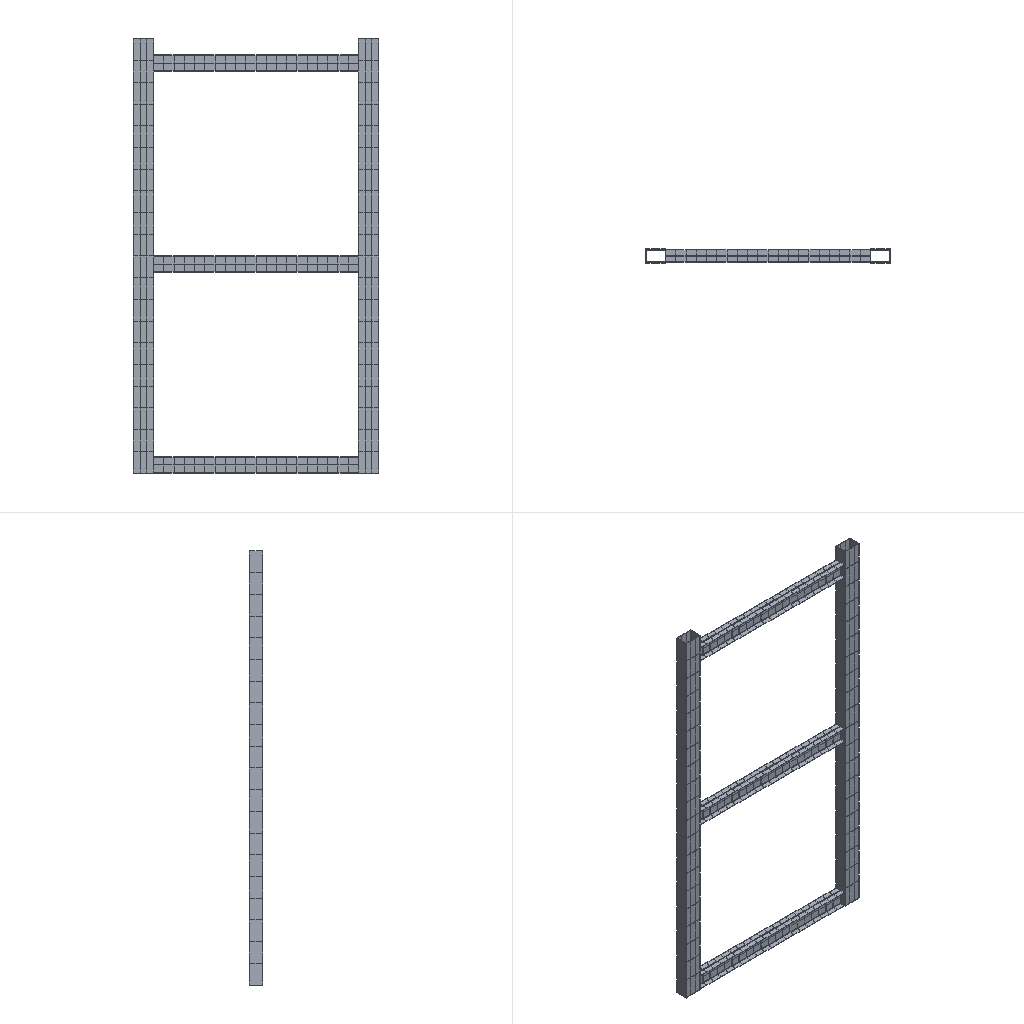Simulation study | abaqus
Set-up summary:
category,name,step,type,value,unit,region
solver,abaqus,,Abaqus/CAE 2024
units,mm-N-s-tonne (MPa),,inferred,E=206000 density=7.85e-09
analysis,Step-1,,static,nlgeom=True; time_period=20
mesh,nodes,,,1807
mesh,elements,,,800
element_type,C3D8R,,,800
material,q335b,,E,206000
material,q335b,,nu,0.3
material,q335b,,density,7.85e-09
material,q335b,,yield,335
material,q335b,,behaviors,plastic
section,q335b,,solid section,,,Set-1
section,q335b,,solid section,,,Set-1
bc,BC-1,initial,encastre,[dofs=ENCASTRE],,_PickedSet31
bc,BC-2,Step-1,displacement,1 [dofs=x],,_PickedSet32
bc,BC-2,Step-1,fixed,"[dofs=rx,rz,y n=3]",,_PickedSet32
contact,CP-1-Part-1-1-liang-1,initial,tie,,,CP-2-liang-1 / CP-1-Part-1-1
contact,CP-1-Part-1-1-lin-2-1-liang-1,initial,tie,,,CP-1-liang-1 / CP-1-Part-1-1-lin-2-1
constraint,coupling,,,1
Abaqus input file, long lists of numbers shortened:
*Heading
** Job name: deck Model name: Model-1-Copy
** Generated by: Abaqus/CAE 2024
*Preprint, echo=NO, model=NO, history=NO, contact=NO
**
** PARTS
**
*Part, name=Part-1
*Node
      1,         300.,         192.,           0.
      2,         300.,         192.,        6484.
** (334 more lines like these left out)
*Element, type=C3D8R
 1,   8,  81,  82,   7,   1,  25,  62,   4
 2,  81,  80,  83,  82,  25,  26,  61,  62
** (158 more lines like these left out)
*Nset, nset=Set-1, generate
   1,  336,    1
*Elset, elset=Set-1, generate
   1,  160,    1
** Section: zhu
*Solid Section, elset=Set-1, material=q335b
,
*End Part
**
*Part, name=liang
*Node
      1,          82.,         237.,           0.
      2,          82.,         237.,        3060.
** (376 more lines like these left out)
*Element, type=C3D8R
 1,   8,  91,  92,   7,   1,  35,  72,   4
 2,  91,  90,  93,  92,  35,  36,  71,  72
** (158 more lines like these left out)
*Nset, nset=Set-1, generate
   1,  378,    1
*Elset, elset=Set-1, generate
   1,  160,    1
** Section: liang
*Solid Section, elset=Set-1, material=q335b
,
*End Part
**
**
** ASSEMBLY
**
*Assembly, name=Assembly
**
*Instance, name=Part-1-1, part=Part-1
*End Instance
**
*Instance, name=liang-1, part=liang
        300.,         12.5,           0.
        300.,         12.5,           0., 300.577, 13.077, 0.5774,         120.
*End Instance
**
*Instance, name=Part-1-1-lin-2-1, part=Part-1
       3360.,           0.,           0.
*End Instance
**
*Instance, name=liang-1-lin-2-1, part=liang
        300.,         12.5,        3000.
        300.,         12.5,        3000., 300.577, 13.077, 3000.577,         120.
*End Instance
**
*Instance, name=liang-1-lin-3-1, part=liang
        300.,         12.5,        6000.
        300.,         12.5,        6000., 300.577, 13.077, 6000.577,         120.
*End Instance
**
*Node
      1,        3510.,         100.,           0.
*Nset, nset=Set-5
 1,
*Nset, nset=m_Set-1
 1,
*Nset, nset=s_Set-1, instance=Part-1-1-lin-2-1
 12, 14, 18, 21
*Nset, nset=s_Set-3, instance=Part-1-1
 12, 14, 18, 21
*Nset, nset=_PickedSet31, internal, instance=Part-1-1
   2,   3,   5,   6,  10,  11,  13,  16,  17,  19,  20,  24, 160, 161, 240, 241
*Nset, nset=_PickedSet31, internal, instance=Part-1-1-lin-2-1
   2,   3,   5,   6,  10,  11,  13,  16,  17,  19,  20,  24, 160, 161, 240, 241
*Elset, elset=_PickedSet31, internal, instance=Part-1-1
  20,  40,  60,  80, 100, 120, 140, 141
*Elset, elset=_PickedSet31, internal, instance=Part-1-1-lin-2-1
  20,  40,  60,  80, 100, 120, 140, 141
*Nset, nset=_PickedSet32, internal
 1,
*Elset, elset=_CP-1-Part-1-1_S2, internal, instance=Part-1-1
   1,   2,   3,   4,   5,   6,   7,   8,   9,  10,  11,  12,  13,  14,  15,  16
  17,  18,  19,  20,  81,  82,  83,  84,  85,  86,  87,  88,  89,  90,  91,  92
** (1 more lines like these left out)
*Elset, elset=_CP-1-Part-1-1_S1, internal, instance=Part-1-1, generate
 61,  80,   1
*Surface, type=ELEMENT, name=CP-1-Part-1-1
_CP-1-Part-1-1_S2, S2
_CP-1-Part-1-1_S1, S1
*Elset, elset=_CP-1-Part-1-1-lin-2-1_S2, internal, instance=Part-1-1-lin-2-1
  21,  22,  23,  24,  25,  26,  27,  28,  29,  30,  31,  32,  33,  34,  35,  36
  37,  38,  39,  40, 141, 142, 143, 144, 145, 146, 147, 148, 149, 150, 151, 152
** (1 more lines like these left out)
*Elset, elset=_CP-1-Part-1-1-lin-2-1_S1, internal, instance=Part-1-1-lin-2-1, generate
 121,  140,    1
*Surface, type=ELEMENT, name=CP-1-Part-1-1-lin-2-1
_CP-1-Part-1-1-lin-2-1_S2, S2
_CP-1-Part-1-1-lin-2-1_S1, S1
*Elset, elset=_CP-1-liang-1_S4, internal, instance=liang-1
  20,  40,  60, 120
*Elset, elset=_CP-1-liang-1_S4, internal, instance=liang-1-lin-2-1
  20,  40,  60, 120
*Elset, elset=_CP-1-liang-1_S4, internal, instance=liang-1-lin-3-1
  20,  40,  60, 120
*Elset, elset=_CP-1-liang-1_S6, internal, instance=liang-1
 61, 81
*Elset, elset=_CP-1-liang-1_S6, internal, instance=liang-1-lin-2-1
 61, 81
*Elset, elset=_CP-1-liang-1_S6, internal, instance=liang-1-lin-3-1
 61, 81
*Elset, elset=_CP-1-liang-1_S3, internal, instance=liang-1
 121, 122
*Elset, elset=_CP-1-liang-1_S3, internal, instance=liang-1-lin-2-1
 121, 122
*Elset, elset=_CP-1-liang-1_S3, internal, instance=liang-1-lin-3-1
 121, 122
*Surface, type=ELEMENT, name=CP-1-liang-1
_CP-1-liang-1_S4, S4
_CP-1-liang-1_S6, S6
_CP-1-liang-1_S3, S3
*Elset, elset=_CP-2-liang-1_S4, internal, instance=liang-1
  80, 100
*Elset, elset=_CP-2-liang-1_S4, internal, instance=liang-1-lin-2-1
  80, 100
*Elset, elset=_CP-2-liang-1_S4, internal, instance=liang-1-lin-3-1
  80, 100
*Elset, elset=_CP-2-liang-1_S6, internal, instance=liang-1
   1,  21,  41, 101
*Elset, elset=_CP-2-liang-1_S6, internal, instance=liang-1-lin-2-1
   1,  21,  41, 101
*Elset, elset=_CP-2-liang-1_S6, internal, instance=liang-1-lin-3-1
   1,  21,  41, 101
*Elset, elset=_CP-2-liang-1_S5, internal, instance=liang-1
 159, 160
*Elset, elset=_CP-2-liang-1_S5, internal, instance=liang-1-lin-2-1
 159, 160
*Elset, elset=_CP-2-liang-1_S5, internal, instance=liang-1-lin-3-1
 159, 160
*Surface, type=ELEMENT, name=CP-2-liang-1
_CP-2-liang-1_S4, S4
_CP-2-liang-1_S6, S6
_CP-2-liang-1_S5, S5
*Elset, elset=__PickedSurf24_S2, internal, instance=Part-1-1-lin-2-1
  21,  22,  23,  24,  25,  26,  27,  28,  29,  30,  31,  32,  33,  34,  35,  36
  37,  38,  39,  40, 141, 142, 143, 144, 145, 146, 147, 148, 149, 150, 151, 152
** (1 more lines like these left out)
*Elset, elset=__PickedSurf24_S1, internal, instance=Part-1-1-lin-2-1, generate
 121,  140,    1
*Surface, type=ELEMENT, name=_PickedSurf24, internal
__PickedSurf24_S2, S2
__PickedSurf24_S1, S1
*Elset, elset=__PickedSurf25_S4, internal, instance=liang-1-lin-2-1
  20,  40,  60, 120
*Elset, elset=__PickedSurf25_S4, internal, instance=liang-1-lin-3-1
  20,  40,  60, 120
*Elset, elset=__PickedSurf25_S6, internal, instance=liang-1-lin-2-1
 61, 81
*Elset, elset=__PickedSurf25_S6, internal, instance=liang-1-lin-3-1
 61, 81
*Elset, elset=__PickedSurf25_S3, internal, instance=liang-1-lin-2-1
 121, 122
*Elset, elset=__PickedSurf25_S3, internal, instance=liang-1-lin-3-1
 121, 122
*Surface, type=ELEMENT, name=_PickedSurf25, internal
__PickedSurf25_S4, S4
__PickedSurf25_S6, S6
__PickedSurf25_S3, S3
*Elset, elset=__PickedSurf30_S4, internal, instance=Part-1-1
 160,
*Elset, elset=__PickedSurf30_S4, internal, instance=Part-1-1-lin-2-1
 160,
*Elset, elset=__PickedSurf30_S6, internal, instance=Part-1-1, generate
   1,  121,   20
*Elset, elset=__PickedSurf30_S6, internal, instance=Part-1-1-lin-2-1, generate
   1,  121,   20
*Surface, type=ELEMENT, name=_PickedSurf30, internal
__PickedSurf30_S4, S4
__PickedSurf30_S6, S6
** Constraint: CP-1-Part-1-1-liang-1
*Tie, name=CP-1-Part-1-1-liang-1, adjust=yes, type=SURFACE TO SURFACE
CP-2-liang-1, CP-1-Part-1-1
** Constraint: CP-1-Part-1-1-lin-2-1-liang-1
*Tie, name=CP-1-Part-1-1-lin-2-1-liang-1, adjust=yes, type=SURFACE TO SURFACE
CP-1-liang-1, CP-1-Part-1-1-lin-2-1
** Constraint: Constraint-1
*Coupling, constraint name=Constraint-1, ref node=m_Set-1, surface=_PickedSurf30
*Kinematic
*End Assembly
*Amplitude, name=Amp-1
             0.,              0.,              1.,              2.,              2.,             -2.,              3.,              4.
             4.,             -4.,              5.,              6.,              6.,             -6.,              7.,             10.
             8.,            -10.
**
** MATERIALS
**
*Material, name=q335b
*Density
 7.85e-09,
*Elastic
206000., 0.3
*Plastic
335.,    0.
410., 0.025
**
** BOUNDARY CONDITIONS
**
** Name: BC-1 Type: Symmetry/Antisymmetry/Encastre
*Boundary
_PickedSet31, ENCASTRE
** ----------------------------------------------------------------
**
** STEP: Step-1
**
*Step, name=Step-1, nlgeom=YES, inc=10000
*Static, stabilize=0.0002, allsdtol=0.05, continue=NO
0.01, 20., 2e-07, 0.5
**
** BOUNDARY CONDITIONS
**
** Name: BC-2 Type: Displacement/Rotation
*Boundary, amplitude=Amp-1
_PickedSet32, 1, 1, 1.
_PickedSet32, 2, 2
_PickedSet32, 4, 4
_PickedSet32, 6, 6
**
** OUTPUT REQUESTS
**
*Restart, write, frequency=0
**
** FIELD OUTPUT: F-Output-1
**
*Output, field, variable=PRESELECT
**
** HISTORY OUTPUT: H-Output-1
**
*Output, history, variable=PRESELECT
*End Step
Results summary:
result,odb.job_status,,,JOB_STATUS_COMPLETED_SUCCESSFULLY,"consistent, unstated (Abaqus has no unit system)"
result,steps[0].procedure,Step-1,,*STATIC,"consistent, unstated (Abaqus has no unit system)"
result,steps[0].time_period,Step-1,,20,"consistent, unstated (Abaqus has no unit system)"
result,steps[0].n_frames,Step-1,,51,"consistent, unstated (Abaqus has no unit system)"
result,steps[0].last_frame.id,Step-1,,50,"consistent, unstated (Abaqus has no unit system)"
result,steps[0].last_frame.value,Step-1,,20,"consistent, unstated (Abaqus has no unit system)"
result,steps[0].last_frame.description,Step-1,,Increment     50: Step Time =    20.00,"consistent, unstated (Abaqus has no unit system)"
result,steps[0].completed,Step-1,,True,"consistent, unstated (Abaqus has no unit system)"
result,steps[0].max_U_magnitude,Step-1,,10.001,"consistent, unstated (Abaqus has no unit system)"
result,steps[0].max_S_mises,Step-1,,69.08,"consistent, unstated (Abaqus has no unit system)"
result,steps[0].RF_sum[1],Step-1,,0.002319,"consistent, unstated (Abaqus has no unit system)"
result,steps[0].RF_sum[2],Step-1,,0.001953,"consistent, unstated (Abaqus has no unit system)"
result,steps[0].RF_sum[3],Step-1,,-0.005859,"consistent, unstated (Abaqus has no unit system)"